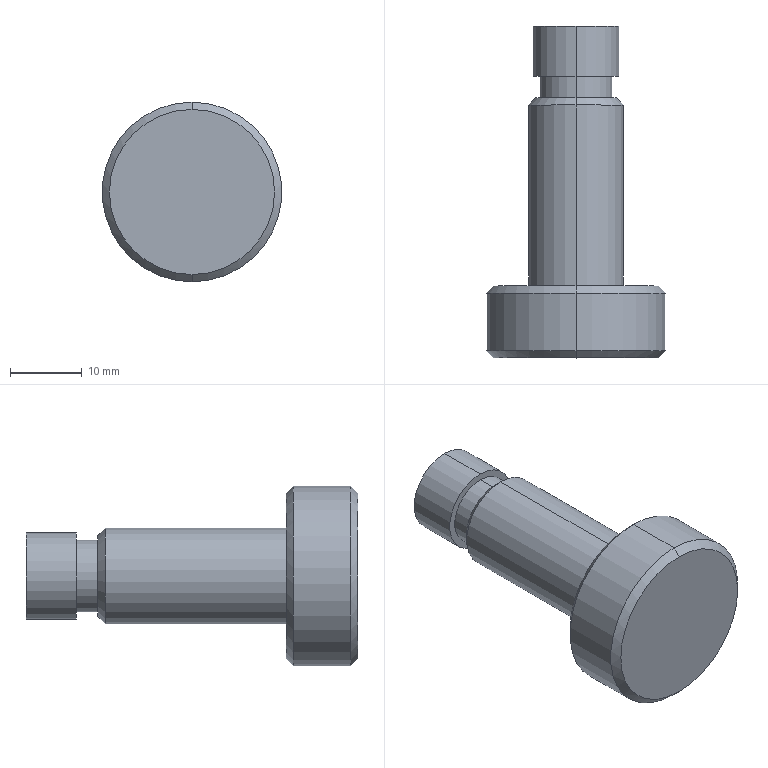Part | SolidWorks | features Chamfer 1, Revolution 1 | 1 solid | 19 faces | box 25 x 46.2 x 25 mm | volume 9480 mm3 | cylinder 8 | cone 6 | plane 5 | commonest cylinder face diameters 10 x2 12 x2 13.3 x2 25 x2
STEP:
#1=CARTESIAN_POINT('',(343.087,66.282,5.65));
#2=VERTEX_POINT('',#1);
#3=CARTESIAN_POINT('',(343.087,66.282,-5.65));
#4=VERTEX_POINT('',#3);
#5=CARTESIAN_POINT('',(343.087,66.282,0.));
#6=DIRECTION('',(0.,1.,0.));
#7=DIRECTION('',(0.,0.,1.));
#8=AXIS2_PLACEMENT_3D('',#5,#6,#7);
#9=CIRCLE('',#8,5.65);
#10=EDGE_CURVE('',#2,#4,#9,.T.);
#11=ORIENTED_EDGE('',*,*,#10,.F.);
#12=CARTESIAN_POINT('',(343.087,65.282,6.65));
#13=VERTEX_POINT('',#12);
#14=CARTESIAN_POINT('',(343.087,65.282,6.65));
#15=DIRECTION('',(0.,-0.7071,0.7071));
#16=VECTOR('',#15,1000.);
#17=LINE('',#14,#16);
#18=EDGE_CURVE('',#2,#13,#17,.T.);
#19=ORIENTED_EDGE('',*,*,#18,.T.);
#20=CARTESIAN_POINT('',(343.087,65.282,-6.65));
#21=VERTEX_POINT('',#20);
#22=CARTESIAN_POINT('',(343.087,65.282,0.));
#23=DIRECTION('',(0.,-1.,0.));
#24=DIRECTION('',(0.,0.,1.));
#25=AXIS2_PLACEMENT_3D('',#22,#23,#24);
#26=CIRCLE('',#25,6.65);
#27=EDGE_CURVE('',#21,#13,#26,.T.);
#28=ORIENTED_EDGE('',*,*,#27,.F.);
#29=CARTESIAN_POINT('',(343.087,65.282,-6.65));
#30=DIRECTION('',(0.,-0.7071,-0.7071));
#31=VECTOR('',#30,1000.);
#32=LINE('',#29,#31);
#33=EDGE_CURVE('',#4,#21,#32,.T.);
#34=ORIENTED_EDGE('',*,*,#33,.F.);
#35=EDGE_LOOP('',(#11,#19,#28,#34));
#36=FACE_OUTER_BOUND('',#35,.T.);
#37=CARTESIAN_POINT('',(343.087,65.282,0.));
#38=DIRECTION('',(0.,-1.,0.));
#39=DIRECTION('',(0.,0.,-1.));
#40=AXIS2_PLACEMENT_3D('',#37,#38,#39);
#41=CONICAL_SURFACE('',#40,6.65,0.7854);
#42=ADVANCED_FACE('',(#36),#41,.T.);
#43=CARTESIAN_POINT('',(343.087,40.082,11.5));
#44=VERTEX_POINT('',#43);
#45=CARTESIAN_POINT('',(343.087,40.082,-11.5));
#46=VERTEX_POINT('',#45);
#47=CARTESIAN_POINT('',(343.087,40.082,0.));
#48=DIRECTION('',(0.,1.,0.));
#49=DIRECTION('',(0.,0.,1.));
#50=AXIS2_PLACEMENT_3D('',#47,#48,#49);
#51=CIRCLE('',#50,11.5);
#52=EDGE_CURVE('',#44,#46,#51,.T.);
#53=ORIENTED_EDGE('',*,*,#52,.F.);
#54=CARTESIAN_POINT('',(343.087,39.082,12.5));
#55=VERTEX_POINT('',#54);
#56=CARTESIAN_POINT('',(343.087,39.082,12.5));
#57=DIRECTION('',(0.,-0.7071,0.7071));
#58=VECTOR('',#57,1000.);
#59=LINE('',#56,#58);
#60=EDGE_CURVE('',#44,#55,#59,.T.);
#61=ORIENTED_EDGE('',*,*,#60,.T.);
#62=CARTESIAN_POINT('',(343.087,39.082,-12.5));
#63=VERTEX_POINT('',#62);
#64=CARTESIAN_POINT('',(343.087,39.082,0.));
#65=DIRECTION('',(0.,-1.,0.));
#66=DIRECTION('',(0.,0.,1.));
#67=AXIS2_PLACEMENT_3D('',#64,#65,#66);
#68=CIRCLE('',#67,12.5);
#69=EDGE_CURVE('',#63,#55,#68,.T.);
#70=ORIENTED_EDGE('',*,*,#69,.F.);
#71=CARTESIAN_POINT('',(343.087,39.082,-12.5));
#72=DIRECTION('',(0.,-0.7071,-0.7071));
#73=VECTOR('',#72,1000.);
#74=LINE('',#71,#73);
#75=EDGE_CURVE('',#46,#63,#74,.T.);
#76=ORIENTED_EDGE('',*,*,#75,.F.);
#77=EDGE_LOOP('',(#53,#61,#70,#76));
#78=FACE_OUTER_BOUND('',#77,.T.);
#79=CARTESIAN_POINT('',(343.087,39.082,0.));
#80=DIRECTION('',(0.,-1.,0.));
#81=DIRECTION('',(0.,0.,-1.));
#82=AXIS2_PLACEMENT_3D('',#79,#80,#81);
#83=CONICAL_SURFACE('',#82,12.5,0.7854);
#84=ADVANCED_FACE('',(#78),#83,.T.);
#85=CARTESIAN_POINT('',(343.087,30.082,-11.5));
#86=VERTEX_POINT('',#85);
#87=CARTESIAN_POINT('',(343.087,30.082,11.5));
#88=VERTEX_POINT('',#87);
#89=CARTESIAN_POINT('',(343.087,30.082,0.));
#90=DIRECTION('',(0.,-1.,0.));
#91=DIRECTION('',(0.,0.,-1.));
#92=AXIS2_PLACEMENT_3D('',#89,#90,#91);
#93=CIRCLE('',#92,11.5);
#94=EDGE_CURVE('',#86,#88,#93,.T.);
#95=ORIENTED_EDGE('',*,*,#94,.F.);
#96=CARTESIAN_POINT('',(343.087,31.082,-12.5));
#97=VERTEX_POINT('',#96);
#98=CARTESIAN_POINT('',(343.087,30.082,-11.5));
#99=DIRECTION('',(0.,0.7071,-0.7071));
#100=VECTOR('',#99,1000.);
#101=LINE('',#98,#100);
#102=EDGE_CURVE('',#86,#97,#101,.T.);
#103=ORIENTED_EDGE('',*,*,#102,.T.);
#104=CARTESIAN_POINT('',(343.087,31.082,12.5));
#105=VERTEX_POINT('',#104);
#106=CARTESIAN_POINT('',(343.087,31.082,0.));
#107=DIRECTION('',(0.,1.,0.));
#108=DIRECTION('',(0.,0.,-1.));
#109=AXIS2_PLACEMENT_3D('',#106,#107,#108);
#110=CIRCLE('',#109,12.5);
#111=EDGE_CURVE('',#105,#97,#110,.T.);
#112=ORIENTED_EDGE('',*,*,#111,.F.);
#113=CARTESIAN_POINT('',(343.087,30.082,11.5));
#114=DIRECTION('',(0.,0.7071,0.7071));
#115=VECTOR('',#114,1000.);
#116=LINE('',#113,#115);
#117=EDGE_CURVE('',#88,#105,#116,.T.);
#118=ORIENTED_EDGE('',*,*,#117,.F.);
#119=EDGE_LOOP('',(#95,#103,#112,#118));
#120=FACE_OUTER_BOUND('',#119,.T.);
#121=CARTESIAN_POINT('',(343.087,30.082,0.));
#122=DIRECTION('',(0.,1.,0.));
#123=DIRECTION('',(0.,0.,1.));
#124=AXIS2_PLACEMENT_3D('',#121,#122,#123);
#125=CONICAL_SURFACE('',#124,11.5,0.7854);
#126=ADVANCED_FACE('',(#120),#125,.T.);
#127=ORIENTED_EDGE('',*,*,#69,.T.);
#128=CARTESIAN_POINT('',(343.087,30.082,12.5));
#129=DIRECTION('',(0.,-1.,0.));
#130=VECTOR('',#129,1000.);
#131=LINE('',#128,#130);
#132=EDGE_CURVE('',#55,#105,#131,.T.);
#133=ORIENTED_EDGE('',*,*,#132,.T.);
#134=ORIENTED_EDGE('',*,*,#111,.T.);
#135=CARTESIAN_POINT('',(343.087,30.082,-12.5));
#136=DIRECTION('',(0.,-1.,0.));
#137=VECTOR('',#136,1000.);
#138=LINE('',#135,#137);
#139=EDGE_CURVE('',#63,#97,#138,.T.);
#140=ORIENTED_EDGE('',*,*,#139,.F.);
#141=EDGE_LOOP('',(#127,#133,#134,#140));
#142=FACE_OUTER_BOUND('',#141,.T.);
#143=CARTESIAN_POINT('',(343.087,30.082,0.));
#144=DIRECTION('',(0.,-1.,0.));
#145=DIRECTION('',(0.,0.,-1.));
#146=AXIS2_PLACEMENT_3D('',#143,#144,#145);
#147=CYLINDRICAL_SURFACE('',#146,12.5);
#148=ADVANCED_FACE('',(#142),#147,.T.);
#149=ORIENTED_EDGE('',*,*,#27,.T.);
#150=CARTESIAN_POINT('',(343.087,40.082,6.65));
#151=VERTEX_POINT('',#150);
#152=CARTESIAN_POINT('',(343.087,30.082,6.65));
#153=DIRECTION('',(0.,-1.,0.));
#154=VECTOR('',#153,1000.);
#155=LINE('',#152,#154);
#156=EDGE_CURVE('',#13,#151,#155,.T.);
#157=ORIENTED_EDGE('',*,*,#156,.T.);
#158=CARTESIAN_POINT('',(343.087,40.082,-6.65));
#159=VERTEX_POINT('',#158);
#160=CARTESIAN_POINT('',(343.087,40.082,0.));
#161=DIRECTION('',(0.,-1.,0.));
#162=DIRECTION('',(0.,0.,-1.));
#163=AXIS2_PLACEMENT_3D('',#160,#161,#162);
#164=CIRCLE('',#163,6.65);
#165=EDGE_CURVE('',#159,#151,#164,.T.);
#166=ORIENTED_EDGE('',*,*,#165,.F.);
#167=CARTESIAN_POINT('',(343.087,30.082,-6.65));
#168=DIRECTION('',(0.,-1.,0.));
#169=VECTOR('',#168,1000.);
#170=LINE('',#167,#169);
#171=EDGE_CURVE('',#21,#159,#170,.T.);
#172=ORIENTED_EDGE('',*,*,#171,.F.);
#173=EDGE_LOOP('',(#149,#157,#166,#172));
#174=FACE_OUTER_BOUND('',#173,.T.);
#175=CARTESIAN_POINT('',(343.087,30.082,0.));
#176=DIRECTION('',(0.,-1.,0.));
#177=DIRECTION('',(0.,0.,-1.));
#178=AXIS2_PLACEMENT_3D('',#175,#176,#177);
#179=CYLINDRICAL_SURFACE('',#178,6.65);
#180=ADVANCED_FACE('',(#174),#179,.T.);
#181=CARTESIAN_POINT('',(343.087,69.282,-5.));
#182=VERTEX_POINT('',#181);
#183=CARTESIAN_POINT('',(343.087,69.282,5.));
#184=VERTEX_POINT('',#183);
#185=CARTESIAN_POINT('',(343.087,69.282,0.));
#186=DIRECTION('',(0.,-1.,0.));
#187=DIRECTION('',(0.,0.,-1.));
#188=AXIS2_PLACEMENT_3D('',#185,#186,#187);
#189=CIRCLE('',#188,5.);
#190=EDGE_CURVE('',#182,#184,#189,.T.);
#191=ORIENTED_EDGE('',*,*,#190,.T.);
#192=CARTESIAN_POINT('',(343.087,66.282,5.));
#193=VERTEX_POINT('',#192);
#194=CARTESIAN_POINT('',(343.087,30.082,5.));
#195=DIRECTION('',(0.,-1.,0.));
#196=VECTOR('',#195,1000.);
#197=LINE('',#194,#196);
#198=EDGE_CURVE('',#184,#193,#197,.T.);
#199=ORIENTED_EDGE('',*,*,#198,.T.);
#200=CARTESIAN_POINT('',(343.087,66.282,-5.));
#201=VERTEX_POINT('',#200);
#202=CARTESIAN_POINT('',(343.087,66.282,0.));
#203=DIRECTION('',(0.,-1.,0.));
#204=DIRECTION('',(0.,0.,-1.));
#205=AXIS2_PLACEMENT_3D('',#202,#203,#204);
#206=CIRCLE('',#205,5.);
#207=EDGE_CURVE('',#201,#193,#206,.T.);
#208=ORIENTED_EDGE('',*,*,#207,.F.);
#209=CARTESIAN_POINT('',(343.087,30.082,-5.));
#210=DIRECTION('',(0.,-1.,0.));
#211=VECTOR('',#210,1000.);
#212=LINE('',#209,#211);
#213=EDGE_CURVE('',#182,#201,#212,.T.);
#214=ORIENTED_EDGE('',*,*,#213,.F.);
#215=EDGE_LOOP('',(#191,#199,#208,#214));
#216=FACE_OUTER_BOUND('',#215,.T.);
#217=CARTESIAN_POINT('',(343.087,30.082,0.));
#218=DIRECTION('',(0.,-1.,0.));
#219=DIRECTION('',(0.,0.,-1.));
#220=AXIS2_PLACEMENT_3D('',#217,#218,#219);
#221=CYLINDRICAL_SURFACE('',#220,5.);
#222=ADVANCED_FACE('',(#216),#221,.T.);
#223=CARTESIAN_POINT('',(343.087,76.282,-6.));
#224=VERTEX_POINT('',#223);
#225=CARTESIAN_POINT('',(343.087,76.282,6.));
#226=VERTEX_POINT('',#225);
#227=CARTESIAN_POINT('',(343.087,76.282,0.));
#228=DIRECTION('',(0.,-1.,0.));
#229=DIRECTION('',(0.,0.,-1.));
#230=AXIS2_PLACEMENT_3D('',#227,#228,#229);
#231=CIRCLE('',#230,6.);
#232=EDGE_CURVE('',#224,#226,#231,.T.);
#233=ORIENTED_EDGE('',*,*,#232,.T.);
#234=CARTESIAN_POINT('',(343.087,69.282,6.));
#235=VERTEX_POINT('',#234);
#236=CARTESIAN_POINT('',(343.087,30.082,6.));
#237=DIRECTION('',(0.,-1.,0.));
#238=VECTOR('',#237,1000.);
#239=LINE('',#236,#238);
#240=EDGE_CURVE('',#226,#235,#239,.T.);
#241=ORIENTED_EDGE('',*,*,#240,.T.);
#242=CARTESIAN_POINT('',(343.087,69.282,-6.));
#243=VERTEX_POINT('',#242);
#244=CARTESIAN_POINT('',(343.087,69.282,0.));
#245=DIRECTION('',(0.,-1.,0.));
#246=DIRECTION('',(0.,0.,-1.));
#247=AXIS2_PLACEMENT_3D('',#244,#245,#246);
#248=CIRCLE('',#247,6.);
#249=EDGE_CURVE('',#243,#235,#248,.T.);
#250=ORIENTED_EDGE('',*,*,#249,.F.);
#251=CARTESIAN_POINT('',(343.087,30.082,-6.));
#252=DIRECTION('',(0.,-1.,0.));
#253=VECTOR('',#252,1000.);
#254=LINE('',#251,#253);
#255=EDGE_CURVE('',#224,#243,#254,.T.);
#256=ORIENTED_EDGE('',*,*,#255,.F.);
#257=EDGE_LOOP('',(#233,#241,#250,#256));
#258=FACE_OUTER_BOUND('',#257,.T.);
#259=CARTESIAN_POINT('',(343.087,30.082,0.));
#260=DIRECTION('',(0.,-1.,0.));
#261=DIRECTION('',(0.,0.,-1.));
#262=AXIS2_PLACEMENT_3D('',#259,#260,#261);
#263=CYLINDRICAL_SURFACE('',#262,6.);
#264=ADVANCED_FACE('',(#258),#263,.T.);
#265=ORIENTED_EDGE('',*,*,#232,.F.);
#266=CARTESIAN_POINT('',(343.087,76.282,0.));
#267=DIRECTION('',(0.,-1.,0.));
#268=DIRECTION('',(0.,0.,-1.));
#269=AXIS2_PLACEMENT_3D('',#266,#267,#268);
#270=CIRCLE('',#269,6.);
#271=EDGE_CURVE('',#226,#224,#270,.T.);
#272=ORIENTED_EDGE('',*,*,#271,.F.);
#273=EDGE_LOOP('',(#265,#272));
#274=FACE_OUTER_BOUND('',#273,.T.);
#275=CARTESIAN_POINT('',(349.087,76.282,0.));
#276=DIRECTION('',(0.,1.,0.));
#277=DIRECTION('',(0.,0.,1.));
#278=AXIS2_PLACEMENT_3D('',#275,#276,#277);
#279=PLANE('',#278);
#280=ADVANCED_FACE('',(#274),#279,.T.);
#281=ORIENTED_EDGE('',*,*,#240,.F.);
#282=ORIENTED_EDGE('',*,*,#271,.T.);
#283=ORIENTED_EDGE('',*,*,#255,.T.);
#284=CARTESIAN_POINT('',(343.087,69.282,0.));
#285=DIRECTION('',(0.,-1.,0.));
#286=DIRECTION('',(0.,0.,-1.));
#287=AXIS2_PLACEMENT_3D('',#284,#285,#286);
#288=CIRCLE('',#287,6.);
#289=EDGE_CURVE('',#235,#243,#288,.T.);
#290=ORIENTED_EDGE('',*,*,#289,.F.);
#291=EDGE_LOOP('',(#281,#282,#283,#290));
#292=FACE_OUTER_BOUND('',#291,.T.);
#293=CARTESIAN_POINT('',(343.087,30.082,0.));
#294=DIRECTION('',(0.,-1.,0.));
#295=DIRECTION('',(0.,0.,-1.));
#296=AXIS2_PLACEMENT_3D('',#293,#294,#295);
#297=CYLINDRICAL_SURFACE('',#296,6.);
#298=ADVANCED_FACE('',(#292),#297,.T.);
#299=ORIENTED_EDGE('',*,*,#249,.T.);
#300=ORIENTED_EDGE('',*,*,#289,.T.);
#301=EDGE_LOOP('',(#299,#300));
#302=FACE_OUTER_BOUND('',#301,.T.);
#303=ORIENTED_EDGE('',*,*,#190,.F.);
#304=CARTESIAN_POINT('',(343.087,69.282,0.));
#305=DIRECTION('',(0.,-1.,0.));
#306=DIRECTION('',(0.,0.,-1.));
#307=AXIS2_PLACEMENT_3D('',#304,#305,#306);
#308=CIRCLE('',#307,5.);
#309=EDGE_CURVE('',#184,#182,#308,.T.);
#310=ORIENTED_EDGE('',*,*,#309,.F.);
#311=EDGE_LOOP('',(#303,#310));
#312=FACE_BOUND('',#311,.T.);
#313=CARTESIAN_POINT('',(349.087,69.282,0.));
#314=DIRECTION('',(0.,-1.,0.));
#315=DIRECTION('',(0.,0.,-1.));
#316=AXIS2_PLACEMENT_3D('',#313,#314,#315);
#317=PLANE('',#316);
#318=ADVANCED_FACE('',(#302,#312),#317,.T.);
#319=ORIENTED_EDGE('',*,*,#198,.F.);
#320=ORIENTED_EDGE('',*,*,#309,.T.);
#321=ORIENTED_EDGE('',*,*,#213,.T.);
#322=CARTESIAN_POINT('',(343.087,66.282,0.));
#323=DIRECTION('',(0.,-1.,0.));
#324=DIRECTION('',(0.,0.,-1.));
#325=AXIS2_PLACEMENT_3D('',#322,#323,#324);
#326=CIRCLE('',#325,5.);
#327=EDGE_CURVE('',#193,#201,#326,.T.);
#328=ORIENTED_EDGE('',*,*,#327,.F.);
#329=EDGE_LOOP('',(#319,#320,#321,#328));
#330=FACE_OUTER_BOUND('',#329,.T.);
#331=CARTESIAN_POINT('',(343.087,30.082,0.));
#332=DIRECTION('',(0.,-1.,0.));
#333=DIRECTION('',(0.,0.,-1.));
#334=AXIS2_PLACEMENT_3D('',#331,#332,#333);
#335=CYLINDRICAL_SURFACE('',#334,5.);
#336=ADVANCED_FACE('',(#330),#335,.T.);
#337=CARTESIAN_POINT('',(343.087,66.282,0.));
#338=DIRECTION('',(0.,1.,0.));
#339=DIRECTION('',(0.,0.,1.));
#340=AXIS2_PLACEMENT_3D('',#337,#338,#339);
#341=CIRCLE('',#340,5.65);
#342=EDGE_CURVE('',#4,#2,#341,.T.);
#343=ORIENTED_EDGE('',*,*,#342,.T.);
#344=ORIENTED_EDGE('',*,*,#10,.T.);
#345=EDGE_LOOP('',(#343,#344));
#346=FACE_OUTER_BOUND('',#345,.T.);
#347=ORIENTED_EDGE('',*,*,#207,.T.);
#348=ORIENTED_EDGE('',*,*,#327,.T.);
#349=EDGE_LOOP('',(#347,#348));
#350=FACE_BOUND('',#349,.T.);
#351=CARTESIAN_POINT('',(348.087,66.282,0.));
#352=DIRECTION('',(0.,1.,0.));
#353=DIRECTION('',(0.,0.,1.));
#354=AXIS2_PLACEMENT_3D('',#351,#352,#353);
#355=PLANE('',#354);
#356=ADVANCED_FACE('',(#346,#350),#355,.T.);
#357=ORIENTED_EDGE('',*,*,#156,.F.);
#358=CARTESIAN_POINT('',(343.087,65.282,0.));
#359=DIRECTION('',(0.,-1.,0.));
#360=DIRECTION('',(0.,0.,1.));
#361=AXIS2_PLACEMENT_3D('',#358,#359,#360);
#362=CIRCLE('',#361,6.65);
#363=EDGE_CURVE('',#13,#21,#362,.T.);
#364=ORIENTED_EDGE('',*,*,#363,.T.);
#365=ORIENTED_EDGE('',*,*,#171,.T.);
#366=CARTESIAN_POINT('',(343.087,40.082,0.));
#367=DIRECTION('',(0.,-1.,0.));
#368=DIRECTION('',(0.,0.,-1.));
#369=AXIS2_PLACEMENT_3D('',#366,#367,#368);
#370=CIRCLE('',#369,6.65);
#371=EDGE_CURVE('',#151,#159,#370,.T.);
#372=ORIENTED_EDGE('',*,*,#371,.F.);
#373=EDGE_LOOP('',(#357,#364,#365,#372));
#374=FACE_OUTER_BOUND('',#373,.T.);
#375=CARTESIAN_POINT('',(343.087,30.082,0.));
#376=DIRECTION('',(0.,-1.,0.));
#377=DIRECTION('',(0.,0.,-1.));
#378=AXIS2_PLACEMENT_3D('',#375,#376,#377);
#379=CYLINDRICAL_SURFACE('',#378,6.65);
#380=ADVANCED_FACE('',(#374),#379,.T.);
#381=CARTESIAN_POINT('',(343.087,40.082,0.));
#382=DIRECTION('',(0.,1.,0.));
#383=DIRECTION('',(0.,0.,1.));
#384=AXIS2_PLACEMENT_3D('',#381,#382,#383);
#385=CIRCLE('',#384,11.5);
#386=EDGE_CURVE('',#46,#44,#385,.T.);
#387=ORIENTED_EDGE('',*,*,#386,.T.);
#388=ORIENTED_EDGE('',*,*,#52,.T.);
#389=EDGE_LOOP('',(#387,#388));
#390=FACE_OUTER_BOUND('',#389,.T.);
#391=ORIENTED_EDGE('',*,*,#165,.T.);
#392=ORIENTED_EDGE('',*,*,#371,.T.);
#393=EDGE_LOOP('',(#391,#392));
#394=FACE_BOUND('',#393,.T.);
#395=CARTESIAN_POINT('',(349.737,40.082,0.));
#396=DIRECTION('',(0.,1.,0.));
#397=DIRECTION('',(0.,0.,1.));
#398=AXIS2_PLACEMENT_3D('',#395,#396,#397);
#399=PLANE('',#398);
#400=ADVANCED_FACE('',(#390,#394),#399,.T.);
#401=ORIENTED_EDGE('',*,*,#132,.F.);
#402=CARTESIAN_POINT('',(343.087,39.082,0.));
#403=DIRECTION('',(0.,-1.,0.));
#404=DIRECTION('',(0.,0.,1.));
#405=AXIS2_PLACEMENT_3D('',#402,#403,#404);
#406=CIRCLE('',#405,12.5);
#407=EDGE_CURVE('',#55,#63,#406,.T.);
#408=ORIENTED_EDGE('',*,*,#407,.T.);
#409=ORIENTED_EDGE('',*,*,#139,.T.);
#410=CARTESIAN_POINT('',(343.087,31.082,0.));
#411=DIRECTION('',(0.,1.,0.));
#412=DIRECTION('',(0.,0.,-1.));
#413=AXIS2_PLACEMENT_3D('',#410,#411,#412);
#414=CIRCLE('',#413,12.5);
#415=EDGE_CURVE('',#97,#105,#414,.T.);
#416=ORIENTED_EDGE('',*,*,#415,.T.);
#417=EDGE_LOOP('',(#401,#408,#409,#416));
#418=FACE_OUTER_BOUND('',#417,.T.);
#419=CARTESIAN_POINT('',(343.087,30.082,0.));
#420=DIRECTION('',(0.,-1.,0.));
#421=DIRECTION('',(0.,0.,-1.));
#422=AXIS2_PLACEMENT_3D('',#419,#420,#421);
#423=CYLINDRICAL_SURFACE('',#422,12.5);
#424=ADVANCED_FACE('',(#418),#423,.T.);
#425=CARTESIAN_POINT('',(343.087,30.082,0.));
#426=DIRECTION('',(0.,-1.,0.));
#427=DIRECTION('',(0.,0.,-1.));
#428=AXIS2_PLACEMENT_3D('',#425,#426,#427);
#429=CIRCLE('',#428,11.5);
#430=EDGE_CURVE('',#88,#86,#429,.T.);
#431=ORIENTED_EDGE('',*,*,#430,.T.);
#432=ORIENTED_EDGE('',*,*,#94,.T.);
#433=EDGE_LOOP('',(#431,#432));
#434=FACE_OUTER_BOUND('',#433,.T.);
#435=CARTESIAN_POINT('',(355.587,30.082,0.));
#436=DIRECTION('',(0.,-1.,0.));
#437=DIRECTION('',(0.,0.,-1.));
#438=AXIS2_PLACEMENT_3D('',#435,#436,#437);
#439=PLANE('',#438);
#440=ADVANCED_FACE('',(#434),#439,.T.);
#441=ORIENTED_EDGE('',*,*,#102,.F.);
#442=ORIENTED_EDGE('',*,*,#430,.F.);
#443=ORIENTED_EDGE('',*,*,#117,.T.);
#444=ORIENTED_EDGE('',*,*,#415,.F.);
#445=EDGE_LOOP('',(#441,#442,#443,#444));
#446=FACE_OUTER_BOUND('',#445,.T.);
#447=CARTESIAN_POINT('',(343.087,30.082,0.));
#448=DIRECTION('',(0.,1.,0.));
#449=DIRECTION('',(0.,0.,1.));
#450=AXIS2_PLACEMENT_3D('',#447,#448,#449);
#451=CONICAL_SURFACE('',#450,11.5,0.7854);
#452=ADVANCED_FACE('',(#446),#451,.T.);
#453=ORIENTED_EDGE('',*,*,#60,.F.);
#454=ORIENTED_EDGE('',*,*,#386,.F.);
#455=ORIENTED_EDGE('',*,*,#75,.T.);
#456=ORIENTED_EDGE('',*,*,#407,.F.);
#457=EDGE_LOOP('',(#453,#454,#455,#456));
#458=FACE_OUTER_BOUND('',#457,.T.);
#459=CARTESIAN_POINT('',(343.087,39.082,0.));
#460=DIRECTION('',(0.,-1.,0.));
#461=DIRECTION('',(0.,0.,-1.));
#462=AXIS2_PLACEMENT_3D('',#459,#460,#461);
#463=CONICAL_SURFACE('',#462,12.5,0.7854);
#464=ADVANCED_FACE('',(#458),#463,.T.);
#465=ORIENTED_EDGE('',*,*,#18,.F.);
#466=ORIENTED_EDGE('',*,*,#342,.F.);
#467=ORIENTED_EDGE('',*,*,#33,.T.);
#468=ORIENTED_EDGE('',*,*,#363,.F.);
#469=EDGE_LOOP('',(#465,#466,#467,#468));
#470=FACE_OUTER_BOUND('',#469,.T.);
#471=CARTESIAN_POINT('',(343.087,65.282,0.));
#472=DIRECTION('',(0.,-1.,0.));
#473=DIRECTION('',(0.,0.,-1.));
#474=AXIS2_PLACEMENT_3D('',#471,#472,#473);
#475=CONICAL_SURFACE('',#474,6.65,0.7854);
#476=ADVANCED_FACE('',(#470),#475,.T.);
#477=CLOSED_SHELL('',(#42,#84,#126,#148,#180,#222,#264,#280,#298,#318,#336,#356,#380,#400,#424,#440,#452,#464,#476));
#478=MANIFOLD_SOLID_BREP('',#477);
#479=CARTESIAN_POINT('',(0.,0.,0.));
#480=DIRECTION('',(0.,0.,1.));
#481=DIRECTION('',(1.,0.,0.));
#482=AXIS2_PLACEMENT_3D('',#479,#480,#481);
#483=(LENGTH_UNIT()NAMED_UNIT(*)SI_UNIT(.MILLI.,.METRE.));
#484=UNCERTAINTY_MEASURE_WITH_UNIT(LENGTH_MEASURE(0.00001),#483,'','');
#485=(NAMED_UNIT(*)PLANE_ANGLE_UNIT()SI_UNIT($,.RADIAN.));
#486=(NAMED_UNIT(*)SI_UNIT($,.STERADIAN.)SOLID_ANGLE_UNIT());
#487=(GEOMETRIC_REPRESENTATION_CONTEXT(3)GLOBAL_UNCERTAINTY_ASSIGNED_CONTEXT((#484))GLOBAL_UNIT_ASSIGNED_CONTEXT((#483,#485,#486))REPRESENTATION_CONTEXT('',''));
#488=ADVANCED_BREP_SHAPE_REPRESENTATION('',(#478,#482),#487);